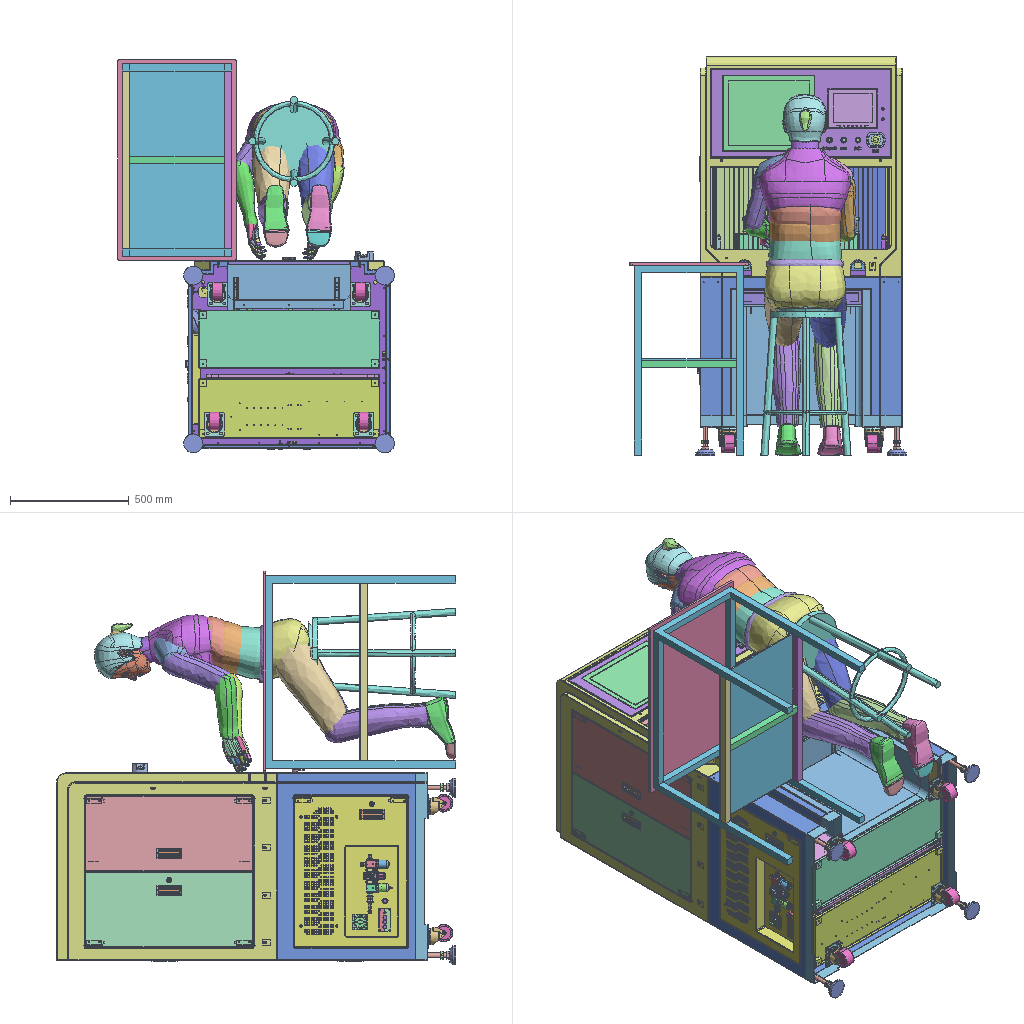Assembly | SolidWorks | 209 different items | 351 placed | box 1166 x 1682 x 1659 mm
Parts list (item | name | quantity | parent item | size | volume | features):
1 | (subassembly) | x1 | - | 263.704 x 74.5 x 59.5 mm | 261559 mm3 | -
2 | (subassembly) | x2 | in 6 | 37.5 x 724 x 636 mm | 879257 mm3 | -
3 | (subassembly) | x1 | in 6 | 37.5 x 764 x 737 mm | 1042688 mm3 | -
4 | (subassembly) | x1 | in 3 | 35.649 x 764 x 379.5 mm | 533274 mm3 | -
5 | (subassembly) | x1 | in 3 | 37.5 x 764 x 367.5 mm | 509414 mm3 | -
6 | (subassembly) | x1 | - | - | 7744813 mm3 | features ReferencePattern 9, LocalLPattern 2
7 | (subassembly) | x2 | in 2 | 35.649 x 724 x 329 mm | 451406 mm3 | -
8 | (subassembly) | x2 | in 2 | 37.5 x 724 x 317 mm | 427850 mm3 | -
9 | (subassembly) | x1 | - | - | 9143617 mm3 | features HoleWzd 1
10 | (subassembly) | x1 | in 9 | 37.5 x 494 x 636 mm | 633113 mm3 | -
11 | (subassembly) | x1 | - | - | 5781926 mm3 | -
12 | (subassembly) | x1 | in 9 | 37.5 x 494 x 731 mm | 708096 mm3 | -
13 | (subassembly) | x1 | - | 851.002 x 954.449 x 1522 mm | 114343551 mm3 | -
14 | (subassembly) | x2 | in 15 | 75 x 75 x 100.5 mm | 180032 mm3 | -
15 | (subassembly) | x1 | in 22 | - | 6635469 mm3 | features CompositeCurve 14, InContextFeatHolder 6, ReferencePattern 5, LocalLPattern 1
16 | (subassembly) | x1 | - | 27.5 x 27.5 x 50 mm | 15432 mm3 | -
17 | (subassembly) | x1 | - | 27.486 x 37 x 27.571 mm | 9512 mm3 | features AEMSimFeature 1
18 | (subassembly) | x1 | - | 27.486 x 37 x 27.571 mm | 9512 mm3 | features AEMSimFeature 1
19 | (subassembly) | x2 | - | 120.002 x 37.222 x 120.002 mm | 118437 mm3 | features AEMSimFeature 1
20 | (subassembly) | x1 | in 22 | - | 7028567 mm3 | -
21 | (subassembly) | x1 | in 20 | - | 7028567 mm3 | features InContextFeatHolder 12
22 | (subassembly) | x1 | - | - | 13967831 mm3 | -
23 | (subassembly) | x1 | in 21 | 66 x 382.5 x 279.882 mm | 1255947 mm3 | features CompositeCurve 1
24 | (subassembly) | x1 | in 25 | 120 x 120 x 447.19 mm | 1943055 mm3 | -
25 | (subassembly) | x1 | in 21 | 150 x 447.19 x 260.95 mm | 4314882 mm3 | features InContextFeatHolder 4, AEMSimFeature 1
26 | (subassembly) | x1 | - | 110 x 110 x 178 mm | 343146 mm3 | -
27 | (subassembly) | x1 | - | 212.5 x 110 x 178 mm | 375386 mm3 | -
28 | (subassembly) | x1 | - | 27.486 x 37 x 27.571 mm | 9512 mm3 | features AEMSimFeature 1
29 | (subassembly) | x1 | in 9 | 513 x 62 x 319 mm | 391027 mm3 | -
30 | (subassembly) | x1 | in 10 | 35.649 x 494 x 329 mm | 327464 mm3 | -
31 | (subassembly) | x1 | in 12 | 35.649 x 494 x 376.5 mm | 364955 mm3 | -
32 | (subassembly) | x1 | in 10 | 37.5 x 494 x 317 mm | 305649 mm3 | -
33 | (subassembly) | x1 | in 23 | 279.882 x 382.5 x 66 mm | 1255947 mm3 | -
34 | (subassembly) | x1 | in 12 | 37.5 x 494 x 364.5 mm | 343141 mm3 | -
35 | (subassembly) | x4 | in 9 | 82 x 108 x 101.5 mm | 268701 mm3 | -
36 | (subassembly) | x1 | in 33 | 129 x 145.682 x 60 mm | 347551 mm3 | -
37 | (subassembly) | x1 | - | - | - | features InContextFeatHolder 2
38 | (subassembly) | x2 | in 9 | 19.1 x 27 x 355.6 mm | 53806 mm3 | features AEMSimFeature 1
39 | (subassembly) | x1 | - | 62 x 132 x 147 mm | 286848 mm3 | -
40 | - | x1 | - | - | - | features RefSurface 13
41 | - | x2 | in 14 | 24 x 24 x 95 mm | 18042 mm3 | features ICE 4, Chamfer 3, HoleWzd 2, Extrusion 1
42 | - | x1 | - | 80 x 64 x 38.5 mm | 66365 mm3 | features BaseBody 1
43 | - | x1 | - | 40 x 40 x 73.5 mm | 58670 mm3 | features ICE 8, CirPattern 2, Chamfer 1, Extrusion 1, MirrorPattern 1, Revolution 1
44 | - | x1 | in 29 | 55 x 52.573 x 12.5 mm | 11112 mm3 | features BaseBody 1, HoleWzd 1
45 | - | x1 | - | 800 x 600 x 10 mm | 4796860 mm3 | features Extrusion 1, Fillet 1, HoleWzd 1
46 | - | x1 | - | 79 x 50 x 11.5 mm | 8238 mm3 | features EdgeFlange 4, HoleWzd 3, Fillet 2, FlatPattern 1, SMBaseFlange 1, SheetMetal 1
47 | - | x1 | in 15 | 40 x 120 x 200 mm | 151570 mm3 | features FlatPattern 1, HoleWzd 1, ICE 1, SMBaseFlange 1, SheetMetal 1
48 | - | x1 | in 15 | 200 x 30 x 20 mm | 113265 mm3 | features Extrusion 1, HoleWzd 1
49 | - | x1 | - | 16.166 x 14 x 25.5 mm | 2115 mm3 | features ICE 1, Revolution 1
50 | - | x1 | - | 16.5 x 51.05 x 30.583 mm | 7205 mm3 | features RevCut 2, Revolution 2, ICE 1
51 | - | x1 | - | - | - | features RefSurface 3
52 | - | x11 | in 4, 5, 7, 8, 9, 30, 31, 32, 34 | 26.5 x 89 x 10.2 mm | 8027 mm3 | features ICE 2, Chamfer 1, Sweep 1
53 | - | x10 | in 4, 7, 30, 31 | 42 x 30.3 x 68.3 mm | 12070 mm3 | features BaseBody 4
54 | - | x11 | in 4, 5, 7, 8, 9, 30, 31, 32, 34 | 26.5 x 89 x 10.2 mm | 8027 mm3 | features ICE 2, Chamfer 1, Sweep 1
55 | - | x4 | in 15 | 30 x 30 x 4.5 mm | 1696 mm3 | features Extrusion 1
56 | - | x4 | in 15 | 75 x 75 x 50 mm | 173343 mm3 | features HoleWzd 2, Extrusion 1, RevCut 1
57 | - | x1 | in 15 | 520 x 157 x 80 mm | 647127 mm3 | features ICE 2, SMWeldBead 2, Cut 1, EdgeFlange 1, Fillet 1, FlatPattern 1, HoleWzd 1, SMBaseFlange 1, SheetMetal 1
58 | - | x1 | in 15 | 520 x 157 x 80 mm | 639490 mm3 | features ICE 3, Cut 2, SMWeldBead 2, EdgeFlange 1, Fillet 1, FlatPattern 1, SMBaseFlange 1, SheetMetal 1
59 | - | x2 | in 15 | 25 x 25 x 420 mm | 181738 mm3 | features ICE 4, Chamfer 2, HoleWzd 2, Extrusion 1
60 | - | x1 | in 9 | 851 x 582 x 791 mm | 1784461 mm3 | features ICE 16, Fillet 6, HoleWzd 2, Extrusion 1, Shell 1
61 | - | x2 | - | 22 x 34 x 300 mm | 181288 mm3 | features Extrusion 1
62 | - | x1 | - | 16 x 1.6 x 16 mm | 219.911 mm3 | features Revolution 1
63 | - | x4 | in 6 | 26.5 x 60 x 14.5 mm | 2856 mm3 | features ICE 2, Chamfer 1, FlatPattern 1, SMBaseFlange 1, SheetMetal 1
64 | - | x2 | in 6 | 378 x 24.5 x 30 mm | 18043 mm3 | features ICE 2, Chamfer 1, FlatPattern 1, SMBaseFlange 1, SheetMetal 1
65 | - | x1 | - | 270 x 29.5 x 60 mm | 28669 mm3 | features ICE 2, Chamfer 1, FlatPattern 1, HoleWzd 1, SMBaseFlange 1, SheetMetal 1
66 | - | x1 | in 6 | 758 x 373 x 23.5 mm | 379988 mm3 | features ICE 12, HoleWzd 3, Fillet 2, Extrusion 1, Shell 1
67 | - | x1 | in 9 | 638 x 478 x 53 mm | 589173 mm3 | features ICE 16, Fillet 4, HoleWzd 4, LPattern 4, Cut 1, Extrusion 1
68 | - | x1 | in 15 | 40 x 120 x 619.772 mm | 529398 mm3 | features ICE 3, Fillet 2, HoleWzd 2, Chamfer 1, EdgeFlange 1, FlatPattern 1, SMBaseFlange 1, SheetMetal 1
69 | - | x1 | in 15 | 40 x 120 x 619.772 mm | 529398 mm3 | features Fillet 2, HoleWzd 2, ICE 2, Chamfer 1, Cut 1, EdgeFlange 1, FlatPattern 1, SMBaseFlange 1, SheetMetal 1
70 | - | x1 | in 9 | 729 x 16 x 537 mm | 887754 mm3 | features HoleWzd 7, ICE 2, LPattern 2, EdgeFlange 1, FlatPattern 1, SMBaseFlange 1, SheetMetal 1
71 | - | x1 | - | 65.5 x 65.5 x 79 mm | 180207 mm3 | features ICE 6, Fillet 3, Chamfer 2, Extrusion 1, HoleWzd 1
72 | - | x1 | - | 24 x 27.713 x 43 mm | 10470 mm3 | features ICE 2, Extrusion 1, Fillet 1
73 | - | x1 | - | 12.277 x 12.254 x 2.1 mm | 135.755 mm3 | features Extrusion 1
74 | - | x2 | in 15 | 535 x 85 x 50 mm | 287832 mm3 | features Extrusion 1
75 | - | x1 | in 6 | 210 x 2 x 210 mm | 88000 mm3 | features Extrusion 1, Fillet 1, HoleWzd 1
76 | - | x1 | - | 40 x 100 x 160 mm | 100089 mm3 | features ICE 2, Chamfer 1, FlatPattern 1, SMBaseFlange 1, SheetMetal 1
77 | - | x1 | - | 48 x 48 x 18 mm | 31644 mm3 | features Extrusion 1
78 | - | x1 | in 21 | 180 x 730 x 60 mm | 1457746 mm3 | features HoleWzd 5, Chamfer 1, Extrusion 1, ICE 1, MirrorPattern 1
79 | - | x11 | in 4, 5, 7, 8, 9, 30, 31, 32, 34 | 42.062 x 107.5 x 14.849 mm | 13665 mm3 | features BaseBody 3
80 | - | x6 | in 5, 8, 9, 32, 34 | 21.6 x 37.5 x 21.6 mm | 6258 mm3 | features BaseBody 1
81 | - | x1 | - | 110 x 110 x 178 mm | 318581 mm3 | features ICE 2, MirrorPattern 1, RevCut 1, Revolution 1
82 | - | x1 | - | 160 x 60 x 10 mm | 92142 mm3 | features HoleWzd 2, Extrusion 1
83 | - | x1 | - | - | - | features RefSurface 5
84 | - | x1 | - | 45 x 45 x 500 mm | 317021 mm3 | features Extrusion 1, HoleWzd 1
85 | - | x2 | in 15 | 25 x 13 x 25 mm | 3768 mm3 | features Extrusion 1
86 | - | x1 | in 25 | 92 x 60 x 144 mm | 769072 mm3 | features HoleWzd 2, Chamfer 1, Extrusion 1
87 | - | x1 | in 25 | 140 x 390.5 x 15 mm | 813690 mm3 | features HoleWzd 7, Extrusion 1, Fillet 1, ICE 1
88 | - | x1 | in 15 | 30 x 20 x 30 mm | 7536 mm3 | features Extrusion 1
89 | - | x2 | in 6 | 825 x 30 x 22 mm | 48151 mm3 | features ICE 3, Chamfer 1, Extrusion 1, Fillet 1, HoleWzd 1
90 | - | x1 | - | 590 x 1000 x 5 mm | 2949750 mm3 | features Chamfer 1, Extrusion 1
91 | - | x1 | - | 790 x 1000 x 5 mm | 3949750 mm3 | features Chamfer 1, Extrusion 1
92 | - | x8 | - | 20 x 6 x 6 mm | 537.381 mm3 | features RefAxis 3, 3DProfileFeature 1, RevCut 1, Revolution 1
93 | - | x2 | in 29 | 20 x 23.481 x 200 mm | 6904 mm3 | features BaseBody 1, ICE 1
94 | - | x1 | in 29 | 513 x 62 x 306.5 mm | 366101 mm3 | features ICE 9, Extrusion 1, Fillet 1, Shell 1
95 | - | x1 | - | 45 x 45 x 1000 mm | 638120 mm3 | features Extrusion 1
96 | - | x1 | in 30 | 20.237 x 477 x 329 mm | 273605 mm3 | features EdgeFlange 6, ICE 5, Chamfer 1, FlatPattern 1, SMBaseFlange 1, SheetMetal 1
97 | - | x1 | in 31 | 20.237 x 477 x 376.5 mm | 311097 mm3 | features EdgeFlange 6, ICE 5, Chamfer 1, FlatPattern 1, SMBaseFlange 1, SheetMetal 1
98 | - | x1 | in 32 | 15 x 477 x 317 mm | 269673 mm3 | features EdgeFlange 4, ICE 4, FlatPattern 1, SMBaseFlange 1, SheetMetal 1
99 | - | x1 | in 34 | 15 x 477 x 364.5 mm | 307164 mm3 | features EdgeFlange 4, ICE 4, FlatPattern 1, SMBaseFlange 1, SheetMetal 1
100 | - | x1 | in 33 | 15 x 17 x 15 mm | 2439 mm3 | features BaseBody 1
101 | - | x1 | in 9 | 475 x 165 x 2 mm | 114873 mm3 | features HoleWzd 2, Chamfer 1, Extrusion 1, ICE 1
102 | - | x1 | in 15 | 120 x 185 x 70 mm | 181748 mm3 | features ICE 6, Chamfer 3, Extrusion 1
103 | - | x1 | - | 45 x 45 x 700 mm | 446684 mm3 | features Extrusion 1
104 | - | x1 | - | 45 x 45 x 545 mm | 347775 mm3 | features Extrusion 1
105 | - | x2 | in 19 | 120.002 x 37.222 x 120.002 mm | 72632 mm3 | features BaseBody 1, ICE 1, Scale 1
106 | - | x1 | in 15 | 90 x 200 x 90 mm | 1142205 mm3 | features ICE 6, Fillet 2, CirPattern 1, Extrusion 1, HoleWzd 1, RefAxis 1
107 | - | x1 | in 33 | 105 x 90 x 52.5 mm | 149012 mm3 | features BaseBody 1
108 | - | x1 | in 22 | 405 x 150 x 5 mm | 303750 mm3 | features Extrusion 1
109 | - | x1 | in 24 | 74 x 74 x 66.99 mm | 341850 mm3 | features BaseBody 24
110 | - | x1 | in 24 | 384.7 x 120 x 120 mm | 1601205 mm3 | features BaseBody 1, ICE 1
111 | - | x2 | in 19 | - | - | features RefSurface 1, Scale 1
112 | - | x2 | in 15 | 66 x 13 x 42 mm | 15219 mm3 | features ICE 3, Fillet 2, Extrusion 1
113 | - | x4 | in 14 | 11 x 35 x 35 mm | 5288 mm3 | features Revolution 6, CirPattern 2, RevCut 2, MirrorPattern 1
114 | - | x2 | in 39 | 40.25 x 51.3 x 11.5 mm | 9114 mm3 | features RefAxis 12, ICE 6, 3DProfileFeature 4, RevCut 2, Extrusion 1, Revolution 1
115 | - | x1 | in 39 | 23.253 x 8.6 x 25 mm | 822.627 mm3 | features RefAxis 3, ICE 2, 3DProfileFeature 1, Revolution 1
116 | - | x1 | in 39 | 40 x 61.6 x 47 mm | 55419 mm3 | features ICE 20, RefAxis 12, 3DProfileFeature 4, RevCut 3, Extrusion 1, Revolution 1
117 | - | x1 | in 39 | 36 x 81 x 36 mm | 24193 mm3 | features RefAxis 3, Revolution 2, 3DProfileFeature 1, ICE 1
118 | - | x2 | in 38 | 9.344 x 19.967 x 355.6 mm | 18790 mm3 | features BaseBody 1, RefAxis 1
119 | - | x1 | in 39 | 18 x 23.5 x 18 mm | 1546 mm3 | features RefAxis 6, 3DProfileFeature 2, Revolution 1
120 | - | x2 | in 39 | 4.9 x 38.3 x 11.5 mm | 1758 mm3 | features RefAxis 9, 3DProfileFeature 3, RevCut 2, Extrusion 1, ICE 1
121 | - | x4 | in 39 | 11 x 7 x 7 mm | 216.302 mm3 | features RefAxis 3, 3DProfileFeature 1, ICE 1, Revolution 1
122 | - | x1 | in 39 | 40 x 110.1 x 47 mm | 56293 mm3 | features ICE 40, RefAxis 9, 3DProfileFeature 3, RevCut 3, Extrusion 1, Revolution 1
123 | - | x1 | in 39 | 36 x 68 x 36 mm | 23842 mm3 | features RefAxis 3, 3DProfileFeature 1, ICE 1, Revolution 1
124 | - | x1 | in 17 | 25 x 37 x 25 mm | 9217 mm3 | features ICE 10, Fillet 2, LPattern 1, Revolution 1
125 | - | x1 | in 18 | 25 x 37 x 25 mm | 9217 mm3 | features ICE 10, Fillet 2, LPattern 1, Revolution 1
126 | - | x2 | in 17, 18 | 26.237 x 28.287 x 2 mm | 294.878 mm3 | features Extrusion 1
127 | - | x1 | in 39 | 15 x 27.1 x 27.1 mm | 10099 mm3 | features ICE 16, RefAxis 9, 3DProfileFeature 3, RevCut 2, Extrusion 1, Revolution 1
128 | - | x1 | in 39 | 40 x 43 x 47 mm | 55436 mm3 | features ICE 27, RefAxis 15, 3DProfileFeature 5, RevCut 2, Extrusion 1, LPattern 1, Revolution 1
129 | - | x1 | in 25 | 150 x 181 x 35 mm | 751527 mm3 | features HoleWzd 2, ICE 2, Chamfer 1, Extrusion 1, Fillet 1
130 | - | x1 | in 39 | 37 x 6.5 x 35.922 mm | 2594 mm3 | features RefAxis 3, 3DProfileFeature 1, ICE 1, Revolution 1
131 | - | x4 | in 39 | 5.512 x 5.512 x 9.5 mm | 81.226 mm3 | features RefAxis 3, 3DProfileFeature 1, ICE 1, Revolution 1
132 | - | x2 | in 39 | 4.984 x 5 x 17.2 mm | 126.363 mm3 | features RefAxis 3, 3DProfileFeature 1, ICE 1, Revolution 1
133 | - | x1 | in 39 | 40 x 46 x 38 mm | 33356 mm3 | features RefAxis 18, ICE 10, 3DProfileFeature 6, Extrusion 1, RevCut 1, Revolution 1
134 | - | x4 | in 39 | 5.5 x 5.5 x 1 mm | 15.412 mm3 | features RefAxis 3, 3DProfileFeature 1, ICE 1, Revolution 1
135 | - | x4 | in 35 | 51 x 75 x 75 mm | 191030 mm3 | features BaseBody 1
136 | - | x4 | in 35 | 82 x 12 x 100 mm | 48810 mm3 | features BaseBody 1
137 | - | x4 | in 35 | 70 x 68.5 x 74 mm | 29160 mm3 | features BaseBody 1
138 | - | x1 | in 1 | 59.5 x 68.85 x 59.5 mm | 56089 mm3 | features ICE 7, Fillet 2, CirPattern 1, Extrusion 1, RevCut 1
139 | - | x1 | in 1 | 50 x 253.304 x 50 mm | 205470 mm3 | features ICE 9, Fillet 2, LPattern 2, Chamfer 1, Dome 1, Extrusion 1, RevCut 1
140 | - | x1 | in 25 | 150 x 64.95 x 35 mm | 37539 mm3 | features Chamfer 1, Extrusion 1, Fillet 1, HoleWzd 1, ICE 1
141 | - | x1 | in 16 | 19.63 x 17.35 x 50 mm | 8637 mm3 | features RefAxis 3, 3DProfileFeature 1, ICE 1, Revolution 1
142 | - | x1 | in 16 | 27.5 x 27.5 x 30 mm | 6795 mm3 | features RefAxis 3, 3DProfileFeature 1, Revolution 1
143 | - | x3 | in 33 | 13.7 x 28.4 x 26 mm | 1939 mm3 | features BaseBody 1
144 | - | x1 | in 33 | 7 x 16 x 25.5 mm | 463.296 mm3 | features BaseBody 1
145 | - | x1 | in 33 | 191 x 44 x 63 mm | 28771 mm3 | features BaseBody 1
146 | - | x1 | in 33 | 188 x 63 x 12 mm | 94885 mm3 | features BaseBody 1
147 | - | x1 | in 33 | 104 x 334 x 40 mm | 423472 mm3 | features BaseBody 1
148 | - | x1 | in 33 | 82.5 x 334 x 8.7 mm | 80216 mm3 | features BaseBody 1
149 | - | x1 | in 33 | 102 x 62.7 x 5 mm | 28999 mm3 | features BaseBody 1
150 | - | x1 | in 33 | 74.5 x 16 x 45 mm | 40163 mm3 | features BaseBody 1
151 | - | x2 | in 38 | 9 x 27 x 355.6 mm | 7594 mm3 | features BaseBody 1, RefAxis 1
152 | - | x1 | in 33 | 74.5 x 23 x 45 mm | 54150 mm3 | features BaseBody 1
153 | - | x1 | in 28 | 26.237 x 28.287 x 2 mm | 294.878 mm3 | features Extrusion 1
154 | - | x1 | in 28 | 25 x 37 x 25 mm | 9217 mm3 | features ICE 10, Fillet 2, LPattern 1, Revolution 1
155 | - | x1 | - | 38.971 x 25 x 45 mm | 24565 mm3 | features Extrusion 1, MirrorPattern 1, RevCut 1
156 | - | x1 | - | 100 x 25 x 5 mm | 10800 mm3 | features Fillet 2, Extrusion 1, HoleWzd 1, ICE 1
157 | - | x1 | - | 100 x 25 x 5 mm | 10800 mm3 | features Fillet 2, Extrusion 1, HoleWzd 1, ICE 1
158 | - | x3 | - | 60 x 42 x 30 mm | 30390 mm3 | features Fillet 2, ICE 2, Chamfer 1, Extrusion 1, HoleWzd 1
159 | - | x1 | - | 384 x 316.5 x 50 mm | 4529826 mm3 | features ICE 2, Chamfer 1, CutThin 1, Extrusion 1, HoleWzd 1, MoveFace 1
160 | - | x1 | - | 202 x 162 x 40 mm | 1013492 mm3 | features BaseBody 1
161 | - | x4 | in 9 | - | - | features RefSurface 3
162 | - | x2 | in 38 | 9 x 27 x 355.6 mm | 7594 mm3 | features BaseBody 1, RefAxis 1
163 | - | x1 | in 36 | 6 x 28.381 x 6 mm | 414.888 mm3 | features BaseBody 1
164 | - | x1 | in 36 | 27.962 x 30.887 x 22.9 mm | 4595 mm3 | features BaseBody 1
165 | - | x1 | in 36 | 45.598 x 29.85 x 36 mm | 13881 mm3 | features BaseBody 1
166 | - | x1 | in 36 | 7.8 x 34.633 x 7.8 mm | 896.959 mm3 | features BaseBody 1
167 | - | x1 | in 36 | 23.7 x 19 x 14.5 mm | 1788 mm3 | features BaseBody 1
168 | - | x1 | in 36 | 129 x 60 x 60 mm | 324718 mm3 | features BaseBody 1
169 | - | x1 | in 36 | 23.7 x 14.55 x 11.2 mm | 1255 mm3 | features BaseBody 1
170 | - | x1 | in 4 | 20.237 x 747 x 379.5 mm | 479415 mm3 | features EdgeFlange 6, ICE 5, Chamfer 1, FlatPattern 1, SMBaseFlange 1, SheetMetal 1
171 | - | x1 | in 5 | 15 x 747 x 367.5 mm | 473438 mm3 | features EdgeFlange 4, ICE 4, FlatPattern 1, SMBaseFlange 1, SheetMetal 1
172 | - | x1 | in 6 | 851 x 930 x 791 mm | 4286500 mm3 | features ICE 38, Fillet 16, HoleWzd 10, Chamfer 1, Cut 1, Extrusion 1, LPattern 1, Shell 1
173 | - | x2 | in 38 | 7.8 x 26 x 355.6 mm | 9914 mm3 | features BaseBody 1, RefAxis 1
174 | - | x2 | in 7 | 20.237 x 707 x 329 mm | 397548 mm3 | features EdgeFlange 6, ICE 5, Chamfer 1, FlatPattern 1, SMBaseFlange 1, SheetMetal 1
175 | - | x2 | in 8 | 15 x 707 x 317 mm | 391874 mm3 | features EdgeFlange 4, ICE 4, FlatPattern 1, SMBaseFlange 1, SheetMetal 1
176 | - | x2 | in 15 | 75 x 75 x 50 mm | 180356 mm3 | features HoleWzd 2, Extrusion 1, ICE 1, RevCut 1
177 | - | x2 | in 14 | 24 x 5 x 24 mm | 1909 mm3 | features Chamfer 1, Extrusion 1, HoleWzd 1
178 | - | x1 | in 15 | 20 x 20 x 448 mm | 119242 mm3 | features ICE 5, Chamfer 1, Cut 1, Extrusion 1
179 | - | x1 | in 15 | 25.008 x 57.316 x 57.728 mm | 22409 mm3 | features HoleWzd 2, Chamfer 1, CirPattern 1, Cut 1, Fillet 1, ICE 1, Revolution 1
180 | - | x1 | in 15 | 25.008 x 57.316 x 57.728 mm | 22718 mm3 | features HoleWzd 2, ICE 2, Chamfer 1, CirPattern 1, Cut 1, Fillet 1, Revolution 1
181 | - | x3 | - | 26 x 27.999 x 7 mm | 2114 mm3 | features ICE 4, Dome 1, Extrusion 1
182 | - | x16 | in 6 | 33 x 33 x 25 mm | 2832 mm3 | features ICE 2, Extrusion 1, Fillet 1
183 | - | x1 | in 13 | - | - | features RefSurface 71
184 | - | x2 | in 38 | 7.8 x 26 x 355.6 mm | 9914 mm3 | features BaseBody 1, RefAxis 1
185 | - | x1 | - | 817 x 20 x 757 mm | 11961283 mm3 | features HoleWzd 10, ICE 5, LPattern 2, Extrusion 1, Fillet 1
186 | - | x2 | - | 22 x 290 x 232.8 mm | 181561 mm3 | features ICE 3, Extrusion 1, LPattern 1, MirrorPattern 1, Revolution 1
187 | - | x2 | - | 22 x 450 x 232.8 mm | 289994 mm3 | features ICE 3, Extrusion 1, LPattern 1, MirrorPattern 1, Revolution 1
188 | - | x1 | in 9 | 589 x 380 x 530 mm | 943074 mm3 | features ICE 9, Fillet 6, HoleWzd 3, Cut 2, ExtruThin 1
189 | - | x1 | in 13 | 850 x 500 x 810 mm | 12634142 mm3 | features ICE 6, Extrusion 1, Fillet 1
190 | - | x2 | in 14 | 75 x 75 x 50 mm | 149506 mm3 | features ICE 2, Extrusion 1, RevCut 1
191 | - | x1 | in 9 | 851 x 50 x 791 mm | 311497 mm3 | features ICE 7, Fillet 5, Extrusion 1, Shell 1
192 | - | x1 | in 9 | 764 x 16 x 252 mm | 477309 mm3 | features HoleWzd 6, LPattern 3, EdgeFlange 1, FlatPattern 1, ICE 1, SMBaseFlange 1, SheetMetal 1
193 | - | x1 | in 9 | 764 x 16 x 244.5 mm | 466147 mm3 | features EdgeFlange 1, FlatPattern 1, HoleWzd 1, ICE 1, SMBaseFlange 1, SheetMetal 1
194 | - | x2 | in 15 | 85 x 45 x 15 mm | 38919 mm3 | features Chamfer 1, Extrusion 1, HoleWzd 1, ICE 1
195 | - | x1 | in 15 | 64.757 x 208.466 x 16.625 mm | 48801 mm3 | features Boss 3, CurvePattern 2, Chamfer 1, CompositeCurve 1, Extrusion 1, MirrorPattern 1, MirrorSolid 1
196 | hex lobular socket head cap screws-8.8 gb | x1 | - | - | - | -
197 | hex thin nuts-grades ab-chamfered gb | x1 | - | - | - | -
198 | plain washers--product grade c gb | x1 | - | - | - | -
199 | spring lock washers--normal type gb | x1 | - | - | - | -
200 | Side Plate-1 | x1 | - | - | - | -
201 | Side Plate-2 | x1 | - | - | - | -
202 | Side Plate-3 | x1 | - | - | - | -
203 | Bottom Cover Plate | x1 | - | - | - | -
204 | Square Tube 1 | x1 | - | - | - | -
205 | Square Tube 5 | x1 | - | - | - | -
206 | Square Tube 6 | x1 | - | - | - | -
207 | Square Tube 7 | x1 | - | - | - | -
208 | Square Tube Welded Frame | x1 | - | - | - | -
209 | Leveling Feet and Casters (subassembly) | x1 | - | - | - | -
Mates (type | each side: item.copy, entity, surface, feature), first 465 of 568 lines:
In the top assembly
Concentric | 185.1 face cylinder M3 Tapped Hole 3 | 181.1 face cylinder Extrude 3 | 2 times
Concentric | 185.1 face cylinder M3 Tapped Hole 3 | 181.2 face cylinder Extrude 3 | 2 times
Coordinate | 185.1 select_type:25 | assembly select_type:11
Coincident | 185.1 face plane Boss-Extrude 1 | 181.3 face plane Extrude 1
Coincident | 185.1 face plane Boss-Extrude 1 | 158.1 face plane Extrude 1
Concentric | 185.1 face cylinder M5 Tapped Hole 2 | 158.1 face cylinder M5 Hex Socket Head Cap Screw Counterbore Hole 1 | 2 times
Width | 181.3 face plane Extrude 1 | 181.3 face plane Extrude 1 | 158.1 face plane Extrude 3 | 158.1 face plane Extrude 3
Concentric | 185.1 face cylinder M3 Tapped Hole 3 | 181.3 face cylinder Extrude 3
Coincident | 185.1 face plane Boss-Extrude 1 | 158.2 face plane Extrude 1
Concentric | 185.1 face cylinder M5 Tapped Hole 2 | 158.2 face cylinder M5 Hex Socket Head Cap Screw Counterbore Hole 1 | 2 times
Coincident | 185.1 face plane Boss-Extrude 1 | 181.1 face plane Extrude 1
Coincident | 185.1 face plane Boss-Extrude 1 | 158.3 face plane Extrude 1
Concentric | 185.1 face cylinder M5 Tapped Hole 2 | 158.3 face cylinder M5 Hex Socket Head Cap Screw Counterbore Hole 1 | 2 times
Coincident | 185.1 face plane Boss-Extrude 1 | 181.2 face plane Extrude 1
Concentric | 185.1 face cylinder Ø6.0 (6) DiameterHole 1 | 92.1 face cylinder Revolve 1
Concentric | 185.1 face cylinder Ø6.0 (6) DiameterHole 1 | 92.2 face cylinder Revolve 1
Concentric | 185.1 face cylinder Ø6.0 (6) DiameterHole 1 | 92.3 face cylinder Revolve 1
Concentric | 185.1 face cylinder Ø6.0 (6) DiameterHole 1 | 92.4 face cylinder Revolve 1
Concentric | 185.1 face cylinder Ø6.0 (6) DiameterHole 2 | 92.5 face cylinder Revolve 1
Concentric | 185.1 face cylinder Ø6.0 (6) DiameterHole 2 | 92.6 face cylinder Revolve 1
Concentric | 185.1 face cylinder Ø6.0 (6) DiameterHole 2 | 92.7 face cylinder Revolve 1
Concentric | 185.1 face cylinder Ø6.0 (6) DiameterHole 2 | 92.8 face cylinder Revolve 1
Coincident | 92.3 face plane Revolve 1 | 92.4 face plane Revolve 1
Coincident | 92.1 face plane Revolve 1 | 92.2 face plane Revolve 1
Coincident | 92.7 face plane Revolve 1 | 92.8 face plane Revolve 1
Coincident | 92.5 face plane Revolve 1 | 92.6 face plane Revolve 1
Coincident | 60.1 face plane | 172.1 face plane Boss-Extrude 1 | 2 times
Coincident | 60.1 face plane | 172.1 face plane Boss-Extrude 2
Coincident | 66.1 face plane Boss-Extrude 1 | 42.1 face plane Import 1
Concentric | 66.1 face cylinder Cut-Extrude 5 | 43.1 face cylinder Boss-Extrude 3
Coincident | 66.1 face plane Boss-Extrude 1 | 43.1 face plane Boss-Extrude 1
Concentric | 43.1 face cylinder Boss-Extrude 1 | 42.1 face cylinder Import 1
Concentric | 66.1 face cylinder Cut-Extrude 5 | 125.1 face cylinder Revolve 1
Coincident | 66.1 face plane Boss-Extrude 1 | 125.1 face plane Revolve 1
Concentric | 66.1 face cylinder Cut-Extrude 5 | 124.1 face cylinder Revolve 1
Coincident | 66.1 face plane Boss-Extrude 1 | 124.1 face plane Revolve 1
Concentric | 66.1 face cylinder Cut-Extrude 5 | 154.1 face cylinder Revolve 1
Coincident | 66.1 face plane Boss-Extrude 1 | 154.1 face plane Revolve 1
Coincident | 186.1 face plane Mirror 1 | 186.2 face plane Mirror 1
Coincident | 186.1 face plane Extrude 3 | 186.2 face plane Extrude 3
Coincident | 186.2 face plane Extrude 1 | 187.1 face plane Extrude 1 | 3 times
Coincident | 186.2 face plane Extrude 3 | 89.1 face plane Boss-Extrude 1
Coincident | 187.1 face plane Extrude 3 | 187.2 face plane Extrude 3
Coincident | 187.1 face plane Mirror 1 | 187.2 face plane Mirror 1
Coincident | 187.2 face plane Extrude 1 | 186.1 face plane Extrude 1
Coincident | 187.2 face plane Extrude 3 | 89.2 face plane Boss-Extrude 1
Width | 187.2 face plane Mirror 1 | 186.1 face plane Mirror 1 | 172.1 face plane Shell 1 | 172.1 face plane Shell 1
Width | 186.1 face plane Extrude 3 | 186.1 face plane Extrude 3 | 89.2 face plane Boss-Extrude 1 | 89.2 face plane Boss-Extrude 1
Coincident | 114.1 face plane Boss-Extrude 1 | 67.1 face plane Boss-Extrude 5
Width | 114.2 face plane Cut-Extrude 1 | 114.2 face plane Cut-Extrude 1 | 67.1 face cylinder M5 Tapped Hole 1
Width | 114.1 face plane Cut-Extrude 1 | 114.1 face plane Cut-Extrude 1 | 67.1 face cylinder M5 Tapped Hole 1
DistanceDim | 50.1 face plane Revolve 2 | 141.1 face plane Revolve 1
Concentric | 141.1 face cylinder Revolve 1 | 50.1 face cylinder Revolve 2
Coincident | 116.1 face plane Boss-Extrude 7 | 141.1 face plane Revolve 1
Concentric | 116.1 face cylinder Cut-Revolve 2 | 141.1 face cylinder Revolve 1
Concentric | 72.1 face cylinder Boss-Extrude 4 | 67.1 face cylinder Cut-Extrude 8
Coincident | 72.1 face plane Boss-Extrude 1 | 67.1 face plane Boss-Extrude 5
Concentric | 49.1 face cylinder Revolve 1 | 67.1 face cylinder Cut-Extrude 9
Coincident | 122.1 face plane Boss-Extrude 5 | 49.1 face plane Revolve 1
Concentric | 122.1 edge | 49.1 face cylinder Revolve 1
Coincident | 71.1 face plane Boss-Extrude 5 | 67.1 face plane Boss-Extrude 5
Concentric | 71.1 face cylinder M4 Tapped Hole 1 | 67.1 face cylinder Ø4.5 (4.5) DiameterHole 1 | 2 times
Coincident | 105.1 face plane Import 1 | 101.1 face plane Boss-Extrude 1
Concentric | 105.1 face cylinder Cut-Extrude 1 | 101.1 face cylinder M4 Tapped Hole 1 | 2 times
Coincident | 105.2 face plane Import 1 | 101.1 face plane Boss-Extrude 1
Concentric | 105.2 face cylinder Cut-Extrude 1 | 101.1 face cylinder M4 Tapped Hole 1 | 2 times
Coincident | 66.1 face plane Boss-Extrude 4 | 159.1 face plane Cut-Extrude-Thin 1
Width | 159.1 face plane Boss-Extrude 1 | 159.1 face plane Boss-Extrude 1 | 66.1 face plane Cut-Extrude 2 | 66.1 face plane Cut-Extrude 2
Width | 66.1 face plane Cut-Extrude 2 | 66.1 face plane Cut-Extrude 2 | 159.1 face plane Boss-Extrude 1 | 159.1 face plane Boss-Extrude 1
Coincident | 159.1 face plane Boss-Extrude 1 | 64.1 face plane Base-Flange 1
Width | 64.1 face plane Cut-Extrude 1 | 64.1 face plane Cut-Extrude 1 | 159.1 face cylinder M5 Tapped Hole 1
Coincident | 159.1 face plane Boss-Extrude 1 | 64.2 face plane Base-Flange 1
Width | 64.2 face plane Cut-Extrude 1 | 64.2 face plane Cut-Extrude 1 | 159.1 face cylinder M5 Tapped Hole 1
Concentric | 156.1 face cylinder M3 Hex Socket Countersunk Screw Countersink Hole 1 | 67.1 face cylinder M3 Tapped Hole 1 | 2 times
Coincident | 156.1 face plane Boss-Extrude 1 | 67.1 face plane Boss-Extrude 5
Coincident | 157.1 face plane Boss-Extrude 1 | 67.1 face plane Boss-Extrude 5
Concentric | 157.1 face cylinder M3 Hex Socket Countersunk Screw Countersink Hole 1 | 67.1 face cylinder M3 Tapped Hole 1 | 2 times
Coincident | 63.1 face plane Base-Flange 1 | 61.1 face plane Boss-Extrude 1 | 3 times
Coincident | 61.1 face plane Boss-Extrude 1 | 63.2 face plane Base-Flange 1 | 2 times
Coincident | 61.2 face plane Boss-Extrude 1 | 63.3 face plane Base-Flange 1 | 3 times
Coincident | 63.4 face plane Base-Flange 1 | 61.2 face plane Boss-Extrude 1 | 3 times
Coincident | 185.1 face cone Ø6.0 (6) DiameterHole 2 | 92.6 edge
Coincident | 185.1 face cone Ø6.0 (6) DiameterHole 2 | 92.8 edge
Coincident | 185.1 face cone Ø6.0 (6) DiameterHole 1 | 92.3 edge
Coincident | 185.1 face cone Ø6.0 (6) DiameterHole 1 | 92.2 edge
Width | 160.1 face plane Import 1 | 160.1 face plane Import 1 | 66.1 face plane Cut-Extrude 3 | 66.1 face plane Cut-Extrude 3 | 2 times
Coincident | 66.1 face plane Boss-Extrude 6 | 160.1 face plane Import 1
Coincident | 66.1 face plane Boss-Extrude 7 | 65.1 face plane Base-Flange 1
Width | 65.1 face plane Base-Flange 1 | 65.1 face plane Base-Flange 1 | 66.1 face plane Cut-Extrude 3 | 66.1 face plane Cut-Extrude 3
DistanceDim | 65.1 face plane Base-Flange 1 | 66.1 face plane Boss-Extrude 5
Concentric | 172.1 face cylinder Cut-Extrude 9 | 138.1 face cone Boss-Extrude 1
Parallel | 172.1 face plane Boss-Extrude 1 | 139.1 face plane Boss-Extrude 9
Coincident | 172.1 face plane Boss-Extrude 33 | 138.1 face plane Boss-Extrude 1
Coincident | 185.1 face plane Boss-Extrude 1 | 58.1 face plane Base-Flange 1
Width | 172.1 face plane Boss-Extrude 3 | 172.1 face plane Boss-Extrude 2 | 68.1 face plane Base-Flange 1 | 69.1 face plane Base-Flange 1
DistanceDim | 57.1 face plane Base-Flange 1 | 172.1 face plane Boss-Extrude 1
Coincident | 161.1 face plane HI_WAL01-D80-M20-L125-001-1-surface2 | 183.1 face plane SS03-1-surface1
Coincident | 172.1 face plane Boss-Extrude 1 | 189.1 face plane Boss-Extrude 1
In subassembly 6
Width | 66.2 face plane Boss-Extrude 1 | 66.2 face plane Boss-Extrude 1 | 172.2 face plane Cut-Extrude 2 | 172.2 face plane Cut-Extrude 2
Width | 172.2 face plane Cut-Extrude 2 | 172.2 face plane Cut-Extrude 2 | 66.2 face plane Boss-Extrude 1 | 66.2 face plane Boss-Extrude 1
Coincident | 172.2 face plane Boss-Extrude 4 | 64.3 face plane Base-Flange 1
Coincident | 172.2 face plane Boss-Extrude 4 | 64.4 face plane Base-Flange 1
Width | 172.2 face plane Cut-Extrude 3 | 172.2 face plane Cut-Extrude 3 | 175.1 face plane Edge-Flange 3 | 174.1 face plane Edge-Flange 3
Width | 172.2 face plane Cut-Extrude 3 | 172.2 face plane Cut-Extrude 3 | 175.1 face plane Edge-Flange 1 | 175.1 face plane Edge-Flange 1
Coincident | 172.2 face plane Boss-Extrude 10 | 175.2 face plane Edge-Flange 5
Width | 172.2 face plane Cut-Extrude 4 | 172.2 face plane Cut-Extrude 4 | 174.2 face plane Edge-Flange 3 | 175.2 face plane Edge-Flange 3
Width | 172.2 face plane Cut-Extrude 4 | 172.2 face plane Cut-Extrude 4 | 175.2 face plane Edge-Flange 1 | 175.2 face plane Edge-Flange 1
Coincident | 172.2 face plane Boss-Extrude 12 | 170.1 face plane Edge-Flange 5
Width | 170.1 face plane Edge-Flange 3 | 171.1 face plane Edge-Flange 3 | 172.2 face plane Cut-Extrude 5 | 172.2 face plane Cut-Extrude 5
Width | 170.1 face plane Edge-Flange 1 | 170.1 face plane Edge-Flange 1 | 172.2 face plane Cut-Extrude 5 | 172.2 face plane Cut-Extrude 5
Coincident | 172.2 face plane Boss-Extrude 8 | 175.1 face plane Edge-Flange 5
Coincident | 172.2 face plane Boss-Extrude 5 | 66.2 face plane Boss-Extrude 1
Width | 172.2 face plane Shell 1 | 172.2 face plane Shell 1 | 89.3 face plane Boss-Extrude 1 | 89.3 face plane Boss-Extrude 1
DistanceDim | 172.2 face plane Shell 1 | 89.3 face plane Boss-Extrude 1
Width | 89.3 face plane Cut-Extrude 1 | 89.3 face plane Cut-Extrude 1 | 172.2 face cylinder M4 Tapped Hole 1
Coincident | 89.3 face plane Boss-Extrude 1 | 89.4 face plane Boss-Extrude 1 | 2 times
Width | 89.4 face plane Cut-Extrude 1 | 89.4 face plane Cut-Extrude 1 | 172.2 face cylinder M4 Tapped Hole 1
Coincident | 63.5 face plane Base-Flange 1 | 63.6 face plane Base-Flange 1 | 2 times
Coincident | 172.2 face plane Boss-Extrude 18 | 63.6 face plane Base-Flange 1 | 2 times
Coincident | 172.2 face plane Boss-Extrude 18 | 63.7 face plane Base-Flange 1 | 2 times
Coincident | 172.2 face plane Boss-Extrude 18 | 63.8 face plane Base-Flange 1 | 3 times
Concentric | 172.2 face cylinder M4 Tapped Hole 5 | 75.1 face cylinder Ø5.0 (5) DiameterHole 1 | 2 times
Coincident | 172.2 face plane Shell 1 | 182.1 face plane Boss-Extrude 1
DistanceDim | 172.2 face plane Boss-Extrude 22 | 182.1 face plane Boss-Extrude 1
DistanceDim | 182.1 face plane Boss-Extrude 1 | 172.2 face plane Shell 1
Coincident | 172.2 face plane Shell 1 | 182.2 face plane Boss-Extrude 1
Coincident | 182.1 face plane Boss-Extrude 1 | 182.2 face plane Boss-Extrude 1 | 2 times
Coincident | 172.2 face plane Shell 1 | 182.3 face plane Boss-Extrude 1
Coincident | 182.4 face plane Boss-Extrude 1 | 182.3 face plane Boss-Extrude 1
DistanceDim | 182.3 face plane Boss-Extrude 1 | 172.2 face plane Shell 1
Coincident | 172.2 face plane Shell 1 | 182.5 face plane Boss-Extrude 1
Coincident | 182.2 face plane Boss-Extrude 1 | 182.5 face plane Boss-Extrude 1
DistanceDim | 172.2 face plane Shell 1 | 182.5 face plane Boss-Extrude 1
Coincident | 182.5 face plane Boss-Extrude 1 | 182.6 face plane Boss-Extrude 1
Coincident | 172.2 face plane Shell 1 | 182.6 face plane Boss-Extrude 1
DistanceDim | 182.6 face plane Boss-Extrude 1 | 182.5 face plane Boss-Extrude 1
Coincident | 172.2 face plane Boss-Extrude 1 | 75.1 face plane Boss-Extrude 1
Coincident | 182.5 face plane Boss-Extrude 1 | 182.7 face plane Boss-Extrude 1
Coincident | 172.2 face plane Shell 1 | 182.7 face plane Boss-Extrude 1
DistanceDim | 182.7 face plane Boss-Extrude 1 | 182.5 face plane Boss-Extrude 1
Coincident | 172.2 face plane Shell 1 | 182.8 face plane Boss-Extrude 1
Coincident | 182.6 face plane Boss-Extrude 1 | 182.8 face plane Boss-Extrude 1
DistanceDim | 182.8 face plane Boss-Extrude 1 | 182.6 face plane Boss-Extrude 1
Coincident | 63.8 face plane Base-Flange 1 | 63.7 face plane Base-Flange 1
Coincident | 63.5 face plane Base-Flange 1 | 63.7 face plane Base-Flange 1
In subassembly 2
Coincident | 174.3 face plane Base-Flange 1 | 175.3 face plane Base-Flange 1
DistanceDim | 175.3 face plane Edge-Flange 1 | 174.3 face plane Edge-Flange 6
Coincident | 174.3 face plane Edge-Flange 1 | 175.3 face plane Edge-Flange 1
In subassembly 8
Coincident | 175.4 face plane Base-Flange 1 | 79.1 face plane Import 3
Width | 79.1 face plane Import 3 | 79.1 face plane Import 3 | 175.4 face plane Cut-Extrude 5 | 175.4 face plane Cut-Extrude 5
Width | 79.1 face plane Import 3 | 79.1 face plane Import 2 | 175.4 face plane Cut-Extrude 5 | 175.4 face plane Cut-Extrude 5
Coincident | 175.4 face plane Base-Flange 1 | 54.1 face plane Boss-Extrude 1
DistanceDim | 175.4 face plane Edge-Flange 1 | 54.1 face plane Boss-Extrude 1
DistanceDim | 54.1 face plane Boss-Extrude 1 | 175.4 face plane Edge-Flange 3
Coincident | 175.4 face plane Base-Flange 1 | 52.1 face plane Boss-Extrude 1
Coincident | 54.1 face plane Boss-Extrude 1 | 52.1 face plane Boss-Extrude 1
DistanceDim | 52.1 face plane Boss-Extrude 1 | 175.4 face plane Edge-Flange 1
Concentric | 175.4 face cylinder Cut-Extrude 5 | 80.1 face cylinder Import 1
Coincident | 175.4 face plane Base-Flange 1 | 80.1 face plane Import 1
Parallel | 175.4 face plane Edge-Flange 5 | 80.1 face plane Import 1
In subassembly 7
Coincident | 174.4 face plane Base-Flange 1 | 79.1 face plane Import 3
Width | 79.1 face plane Import 3 | 79.1 face plane Import 3 | 174.4 face plane Cut-Extrude 5 | 174.4 face plane Cut-Extrude 5
Width | 79.1 face plane Import 3 | 79.1 face plane Import 2 | 174.4 face plane Cut-Extrude 5 | 174.4 face plane Cut-Extrude 5
Coincident | 174.4 face plane Base-Flange 1 | 53.1 face plane Import 9
Coincident | 174.4 face plane Edge-Flange 6 | 53.1 face plane Import 9
Coincident | 174.4 face plane Cut-Extrude 3 | 53.1 face plane Import 9
Coincident | 53.1 face plane Import 10 | 53.2 face plane Import 10
Coincident | 174.4 face plane Edge-Flange 6 | 53.2 face plane Import 9
Coincident | 174.4 face plane Cut-Extrude 3 | 53.2 face plane Import 9
Coincident | 174.4 face plane Base-Flange 1 | 54.1 face plane Boss-Extrude 1
DistanceDim | 174.4 face plane Edge-Flange 1 | 54.1 face plane Boss-Extrude 1
DistanceDim | 54.1 face plane Boss-Extrude 1 | 174.4 face plane Edge-Flange 3
Coincident | 174.4 face plane Base-Flange 1 | 52.1 face plane Boss-Extrude 1
Coincident | 54.1 face plane Boss-Extrude 1 | 52.1 face plane Boss-Extrude 1
DistanceDim | 52.1 face plane Boss-Extrude 1 | 174.4 face plane Edge-Flange 1
In subassembly 3
Coincident | 170.2 face plane Base-Flange 1 | 171.2 face plane Base-Flange 1
DistanceDim | 171.2 face plane Edge-Flange 1 | 170.2 face plane Edge-Flange 6
Coincident | 170.2 face plane Edge-Flange 1 | 171.2 face plane Edge-Flange 1
In subassembly 5
Coincident | 171.3 face plane Base-Flange 1 | 79.1 face plane Import 3
Width | 79.1 face plane Import 3 | 79.1 face plane Import 3 | 171.3 face plane Cut-Extrude 5 | 171.3 face plane Cut-Extrude 5
Width | 79.1 face plane Import 3 | 79.1 face plane Import 2 | 171.3 face plane Cut-Extrude 5 | 171.3 face plane Cut-Extrude 5
Coincident | 171.3 face plane Base-Flange 1 | 54.1 face plane Boss-Extrude 1
DistanceDim | 171.3 face plane Edge-Flange 1 | 54.1 face plane Boss-Extrude 1
DistanceDim | 54.1 face plane Boss-Extrude 1 | 171.3 face plane Edge-Flange 3
Coincident | 171.3 face plane Base-Flange 1 | 52.1 face plane Boss-Extrude 1
Coincident | 54.1 face plane Boss-Extrude 1 | 52.1 face plane Boss-Extrude 1
DistanceDim | 52.1 face plane Boss-Extrude 1 | 171.3 face plane Edge-Flange 1
Concentric | 171.3 face cylinder Cut-Extrude 5 | 80.1 face cylinder Import 1
Coincident | 171.3 face plane Base-Flange 1 | 80.1 face plane Import 1
Parallel | 171.3 face plane Edge-Flange 5 | 80.1 face plane Import 1
In subassembly 4
Coincident | 170.3 face plane Base-Flange 1 | 79.1 face plane Import 3
Width | 79.1 face plane Import 3 | 79.1 face plane Import 3 | 170.3 face plane Cut-Extrude 5 | 170.3 face plane Cut-Extrude 5
Width | 79.1 face plane Import 3 | 79.1 face plane Import 2 | 170.3 face plane Cut-Extrude 5 | 170.3 face plane Cut-Extrude 5
Coincident | 170.3 face plane Base-Flange 1 | 53.1 face plane Import 9
Coincident | 170.3 face plane Edge-Flange 6 | 53.1 face plane Import 9
Coincident | 170.3 face plane Cut-Extrude 3 | 53.1 face plane Import 9
Coincident | 53.1 face plane Import 10 | 53.2 face plane Import 10
Coincident | 170.3 face plane Edge-Flange 6 | 53.2 face plane Import 9
Coincident | 170.3 face plane Cut-Extrude 3 | 53.2 face plane Import 9
Coincident | 170.3 face plane Base-Flange 1 | 54.1 face plane Boss-Extrude 1
DistanceDim | 170.3 face plane Edge-Flange 1 | 54.1 face plane Boss-Extrude 1
DistanceDim | 54.1 face plane Boss-Extrude 1 | 170.3 face plane Edge-Flange 3
Coincident | 170.3 face plane Base-Flange 1 | 52.1 face plane Boss-Extrude 1
Coincident | 54.1 face plane Boss-Extrude 1 | 52.1 face plane Boss-Extrude 1
DistanceDim | 52.1 face plane Boss-Extrude 1 | 170.3 face plane Edge-Flange 1
In subassembly 9
Coincident | 188.1 face plane Extrude-Thin 1 | 60.2 face plane | 2 times
Width | 94.1 face plane Boss-Extrude 1 | 94.1 face plane Boss-Extrude 1 | 188.1 face plane Cut-Extrude 5 | 188.1 face plane Cut-Extrude 5
LimitDistanceDim | 188.1 face plane Boss-Extrude 10 | 94.1 face plane Boss-Extrude 1
Coincident | 188.1 face plane Boss-Extrude 10 | 162.1 face plane Import 1
Coincident | 188.1 face plane Boss-Extrude 10 | 162.2 face plane Import 1
Coincident | 162.1 face plane Import 1 | 162.2 face plane Import 1
DistanceDim | 151.1 face plane Import 1 | 151.2 face plane Import 1
DistanceDim | 151.1 face plane Import 1 | 94.1 face plane Boss-Extrude 2
Coincident | 151.2 face plane Import 1 | 94.1 face plane Boss-Extrude 2
Coincident | 96.1 face plane Edge-Flange 5 | 60.2 face plane
DistanceDim | 96.1 face plane Edge-Flange 1 | 60.2 face plane
DistanceDim | 96.1 face plane Edge-Flange 3 | 60.2 face plane
Coincident | 97.1 face plane Edge-Flange 5 | 60.2 face plane
DistanceDim | 97.1 face plane Edge-Flange 1 | 60.2 face plane
DistanceDim | 60.2 face plane | 97.1 face plane Edge-Flange 3
Coincident | 60.2 face plane | 191.1 face plane Boss-Extrude 1
Width | 67.2 face plane Boss-Extrude 1 | 67.2 face plane Boss-Extrude 1 | 60.2 face plane | 60.2 face plane
Width | 60.2 face plane | 60.2 face plane | 67.2 face plane Boss-Extrude 1 | 67.2 face plane Boss-Extrude 1
Coincident | 60.2 face plane | 67.2 face plane Boss-Extrude 2
Coincident | 67.2 face plane Boss-Extrude 1 | 79.1 face plane Import 3
Width | 79.1 face plane Import 3 | 79.1 face plane Import 3 | 67.2 face plane Cut-Extrude 4 | 67.2 face plane Cut-Extrude 4
Width | 67.2 face plane Cut-Extrude 4 | 67.2 face plane Cut-Extrude 4 | 79.1 face plane Import 2 | 79.1 face plane Import 3
Concentric | 67.2 face cylinder Cut-Extrude 3 | 80.1 face cylinder Import 1
Coincident | 67.2 face plane Boss-Extrude 1 | 80.1 face plane Import 1
Coincident | 67.2 face plane Boss-Extrude 1 | 52.1 face plane Boss-Extrude 1
Concentric | 67.2 face cylinder Cut-Extrude 1 | 52.1 face cylinder Sweep 1
DistanceDim | 52.1 face plane Boss-Extrude 1 | 67.2 face plane Boss-Extrude 2
Coincident | 67.2 face plane Boss-Extrude 1 | 54.1 face plane Boss-Extrude 1
Concentric | 67.2 face cylinder Cut-Extrude 2 | 54.1 face cylinder Sweep 1
DistanceDim | 54.1 face plane Boss-Extrude 1 | 67.2 face plane Boss-Extrude 3
Coincident | 67.2 face plane Boss-Extrude 6 | 101.2 face plane Boss-Extrude 1
Concentric | 67.2 face cylinder M4 Tapped Hole 1 | 101.2 face cylinder Ø5.0 (5) DiameterHole 1 | 2 times
Coincident | 161.2 face plane HI_WAL01-D80-M20-L125-001-1-surface2 | 161.3 face plane HI_WAL01-D80-M20-L125-001-1-surface2
Coincident | 161.3 face plane HI_WAL01-D80-M20-L125-001-1-surface2 | 161.4 face plane HI_WAL01-D80-M20-L125-001-1-surface2
Coincident | 161.4 face plane HI_WAL01-D80-M20-L125-001-1-surface2 | 161.5 face plane HI_WAL01-D80-M20-L125-001-1-surface2
In subassembly 10
Coincident | 96.2 face plane Base-Flange 1 | 98.1 face plane Base-Flange 1
DistanceDim | 98.1 face plane Edge-Flange 1 | 96.2 face plane Edge-Flange 6
Coincident | 96.2 face plane Edge-Flange 1 | 98.1 face plane Edge-Flange 1
In subassembly 30
Coincident | 96.3 face plane Base-Flange 1 | 79.1 face plane Import 3
Width | 79.1 face plane Import 3 | 79.1 face plane Import 3 | 96.3 face plane Cut-Extrude 5 | 96.3 face plane Cut-Extrude 5
Width | 79.1 face plane Import 3 | 79.1 face plane Import 2 | 96.3 face plane Cut-Extrude 5 | 96.3 face plane Cut-Extrude 5
Coincident | 96.3 face plane Base-Flange 1 | 53.1 face plane Import 9
Coincident | 96.3 face plane Edge-Flange 6 | 53.1 face plane Import 9
Coincident | 96.3 face plane Cut-Extrude 3 | 53.1 face plane Import 9
Coincident | 53.1 face plane Import 10 | 53.2 face plane Import 10
Coincident | 96.3 face plane Edge-Flange 6 | 53.2 face plane Import 9
Coincident | 96.3 face plane Cut-Extrude 3 | 53.2 face plane Import 9
Coincident | 96.3 face plane Base-Flange 1 | 54.1 face plane Boss-Extrude 1
DistanceDim | 96.3 face plane Edge-Flange 1 | 54.1 face plane Boss-Extrude 1
DistanceDim | 54.1 face plane Boss-Extrude 1 | 96.3 face plane Edge-Flange 3
Coincident | 96.3 face plane Base-Flange 1 | 52.1 face plane Boss-Extrude 1
Coincident | 54.1 face plane Boss-Extrude 1 | 52.1 face plane Boss-Extrude 1
DistanceDim | 52.1 face plane Boss-Extrude 1 | 96.3 face plane Edge-Flange 1
In subassembly 32
Coincident | 98.2 face plane Base-Flange 1 | 79.1 face plane Import 3
Width | 79.1 face plane Import 3 | 79.1 face plane Import 3 | 98.2 face plane Cut-Extrude 5 | 98.2 face plane Cut-Extrude 5
Width | 79.1 face plane Import 3 | 79.1 face plane Import 2 | 98.2 face plane Cut-Extrude 5 | 98.2 face plane Cut-Extrude 5
Coincident | 98.2 face plane Base-Flange 1 | 54.1 face plane Boss-Extrude 1
DistanceDim | 98.2 face plane Edge-Flange 1 | 54.1 face plane Boss-Extrude 1
DistanceDim | 54.1 face plane Boss-Extrude 1 | 98.2 face plane Edge-Flange 3
Coincident | 98.2 face plane Base-Flange 1 | 52.1 face plane Boss-Extrude 1
Coincident | 54.1 face plane Boss-Extrude 1 | 52.1 face plane Boss-Extrude 1
DistanceDim | 52.1 face plane Boss-Extrude 1 | 98.2 face plane Edge-Flange 1
Concentric | 98.2 face cylinder Cut-Extrude 5 | 80.1 face cylinder Import 1
Coincident | 98.2 face plane Base-Flange 1 | 80.1 face plane Import 1
Parallel | 98.2 face plane Edge-Flange 5 | 80.1 face plane Import 1
In subassembly 38
DistanceDim | 184.1 face plane Import 1 | 118.1 face plane Import 1
DistanceDim | 151.3 face plane Import 1 | 184.1 face plane Import 1
DistanceDim | 173.1 face plane Import 1 | 118.1 face plane Import 1
DistanceDim | 162.3 face plane Import 1 | 173.1 face plane Import 1
Coincident | 118.1 plane | 184.1 plane
Coincident | 118.1 plane | 151.3 plane
Coincident | 118.1 plane | 173.1 plane
Coincident | 118.1 plane | 162.3 plane
Coincident | 151.3 face plane Import 1 | 184.1 face plane Import 1
Coincident | 162.3 face plane Import 1 | 173.1 face plane Import 1
LimitDistanceDim | 118.1 face plane Import 1 | 184.1 face plane Import 1
LimitDistanceDim | 151.3 face plane Import 1 | 162.3 face plane Import 1
In subassembly 12
Coincident | 97.2 face plane Base-Flange 1 | 99.1 face plane Base-Flange 1
DistanceDim | 99.1 face plane Edge-Flange 1 | 97.2 face plane Edge-Flange 6
Coincident | 97.2 face plane Edge-Flange 1 | 99.1 face plane Edge-Flange 1
In subassembly 34
Coincident | 99.2 face plane Base-Flange 1 | 79.1 face plane Import 3
Width | 79.1 face plane Import 3 | 79.1 face plane Import 3 | 99.2 face plane Cut-Extrude 5 | 99.2 face plane Cut-Extrude 5
Width | 79.1 face plane Import 3 | 79.1 face plane Import 2 | 99.2 face plane Cut-Extrude 5 | 99.2 face plane Cut-Extrude 5
Coincident | 99.2 face plane Base-Flange 1 | 54.1 face plane Boss-Extrude 1
DistanceDim | 99.2 face plane Edge-Flange 1 | 54.1 face plane Boss-Extrude 1
DistanceDim | 54.1 face plane Boss-Extrude 1 | 99.2 face plane Edge-Flange 3
Coincident | 99.2 face plane Base-Flange 1 | 52.1 face plane Boss-Extrude 1
Coincident | 54.1 face plane Boss-Extrude 1 | 52.1 face plane Boss-Extrude 1
DistanceDim | 52.1 face plane Boss-Extrude 1 | 99.2 face plane Edge-Flange 1
Concentric | 99.2 face cylinder Cut-Extrude 5 | 80.1 face cylinder Import 1
Coincident | 99.2 face plane Base-Flange 1 | 80.1 face plane Import 1
Parallel | 99.2 face plane Edge-Flange 5 | 80.1 face plane Import 1
In subassembly 31
Coincident | 97.3 face plane Base-Flange 1 | 79.1 face plane Import 3
Width | 79.1 face plane Import 3 | 79.1 face plane Import 3 | 97.3 face plane Cut-Extrude 5 | 97.3 face plane Cut-Extrude 5
Width | 79.1 face plane Import 3 | 79.1 face plane Import 2 | 97.3 face plane Cut-Extrude 5 | 97.3 face plane Cut-Extrude 5
Coincident | 97.3 face plane Base-Flange 1 | 53.1 face plane Import 9
Coincident | 97.3 face plane Edge-Flange 6 | 53.1 face plane Import 9
Coincident | 97.3 face plane Cut-Extrude 3 | 53.1 face plane Import 9
Coincident | 53.1 face plane Import 10 | 53.2 face plane Import 10
Coincident | 97.3 face plane Edge-Flange 6 | 53.2 face plane Import 9
Coincident | 97.3 face plane Cut-Extrude 3 | 53.2 face plane Import 9
Coincident | 97.3 face plane Base-Flange 1 | 54.1 face plane Boss-Extrude 1
DistanceDim | 97.3 face plane Edge-Flange 1 | 54.1 face plane Boss-Extrude 1
DistanceDim | 54.1 face plane Boss-Extrude 1 | 97.3 face plane Edge-Flange 3
Coincident | 97.3 face plane Base-Flange 1 | 52.1 face plane Boss-Extrude 1
Coincident | 54.1 face plane Boss-Extrude 1 | 52.1 face plane Boss-Extrude 1
DistanceDim | 52.1 face plane Boss-Extrude 1 | 97.3 face plane Edge-Flange 1
In subassembly 29
Coincident | 94.2 face plane Boss-Extrude 2 | 93.1 face plane Import 1
Coincident | 94.2 face plane Boss-Extrude 2 | 93.2 face plane Import 1
Coincident | 93.1 face plane Import 1 | 93.2 face plane Import 1
DistanceDim | 93.2 face plane Import 1 | 93.1 face plane Import 1
DistanceDim | 94.2 face plane Boss-Extrude 2 | 93.1 face plane Import 1
DistanceDim | 93.1 face plane Import 1 | 94.2 face plane Boss-Extrude 2
Concentric | 94.2 face cylinder Cut-Extrude 6 | 44.1 face cylinder M4 Tapped Hole 1 | 2 times
Coincident | 94.2 face plane Boss-Extrude 1 | 44.1 face plane Import 9
In subassembly 1
Coordinate | 138.2 select_type:25 | 1.1 select_type:11
Concentric | 138.2 face cylinder Boss-Extrude 5 | 139.2 face cylinder Boss-Extrude 9
Coincident | 138.2 face plane Boss-Extrude 5 | 139.2 face plane Boss-Extrude 9
PlanarAngleDim | 139.2 plane | 1.1 plane
In subassembly 28
Concentric | 154.2 face cylinder Revolve 1 | 153.1 face cylinder Boss-Extrude 1
DistanceDim | 154.2 face plane Revolve 1 | 153.1 face plane Boss-Extrude 1
In subassembly 18
Concentric | 125.2 face cylinder Revolve 1 | 126.1 face cylinder Boss-Extrude 1
DistanceDim | 125.2 face plane Revolve 1 | 126.1 face plane Boss-Extrude 1
In subassembly 39
DistanceDim | 127.1 plane | 128.1 plane
Coincident | 128.1 axis | 127.1 axis
PlanarAngleDim | 127.1 plane | 128.1 plane
DistanceDim | 132.1 plane | 127.1 plane
Coincident | 127.1 axis | 132.1 axis | 3 times
PlanarAngleDim | 132.1 plane | 127.1 plane
DistanceDim | 132.2 plane | 127.1 plane
Coincident | 127.1 axis | 132.2 axis | 3 times
PlanarAngleDim | 132.2 plane | 127.1 plane
DistanceDim | 133.1 plane | 128.1 plane
Coincident | 128.1 axis | 133.1 axis | 3 times
PlanarAngleDim | 133.1 plane | 128.1 plane
DistanceDim | 130.1 plane | 133.1 plane
Coincident | 133.1 axis | 130.1 axis | 3 times
PlanarAngleDim | 130.1 plane | 133.1 plane
DistanceDim | 134.1 plane | 133.1 plane
Coincident | 133.1 axis | 134.1 axis | 3 times
PlanarAngleDim | 134.1 plane | 133.1 plane
DistanceDim | 134.2 plane | 133.1 plane
Coincident | 133.1 axis | 134.2 axis | 3 times
PlanarAngleDim | 134.2 plane | 133.1 plane
DistanceDim | 134.3 plane | 133.1 plane
Coincident | 133.1 axis | 134.3 axis | 3 times
PlanarAngleDim | 134.3 plane | 133.1 plane
DistanceDim | 134.4 plane | 133.1 plane
Coincident | 133.1 axis | 134.4 axis | 3 times
PlanarAngleDim | 134.4 plane | 133.1 plane
DistanceDim | 131.1 plane | 133.1 plane
Coincident | 133.1 axis | 131.1 axis | 3 times
PlanarAngleDim | 131.1 plane | 133.1 plane
DistanceDim | 131.2 plane | 133.1 plane
Coincident | 133.1 axis | 131.2 axis | 3 times
PlanarAngleDim | 131.2 plane | 133.1 plane
DistanceDim | 131.3 plane | 133.1 plane
Coincident | 133.1 axis | 131.3 axis | 3 times
PlanarAngleDim | 131.3 plane | 133.1 plane
DistanceDim | 131.4 plane | 133.1 plane
Coincident | 133.1 axis | 131.4 axis | 3 times
PlanarAngleDim | 131.4 plane | 133.1 plane
DistanceDim | 114.3 plane | 128.1 plane
Coincident | 128.1 axis | 114.3 axis | 3 times
PlanarAngleDim | 114.3 plane | 128.1 plane
DistanceDim | 122.2 plane | 114.3 plane
Coincident | 114.3 axis | 122.2 axis | 3 times
PlanarAngleDim | 122.2 plane | 114.3 plane
DistanceDim | 123.1 plane | 122.2 plane
Coincident | 122.2 axis | 123.1 axis | 3 times
PlanarAngleDim | 123.1 plane | 122.2 plane
DistanceDim | 120.1 plane | 114.3 plane
Coincident | 114.3 axis | 120.1 axis | 3 times
PlanarAngleDim | 120.1 plane | 114.3 plane
DistanceDim | 121.1 plane | 120.1 plane
Coincident | 120.1 axis | 121.1 axis | 3 times
PlanarAngleDim | 121.1 plane | 120.1 plane
DistanceDim | 121.2 plane | 120.1 plane
Coincident | 120.1 axis | 121.2 axis | 3 times
PlanarAngleDim | 121.2 plane | 120.1 plane
DistanceDim | 114.4 plane | 128.1 plane
Coincident | 128.1 axis | 114.4 axis | 3 times
PlanarAngleDim | 114.4 plane | 128.1 plane
DistanceDim | 116.2 plane | 114.4 plane
Coincident | 114.4 axis | 116.2 axis | 3 times
PlanarAngleDim | 116.2 plane | 114.4 plane
DistanceDim | 119.1 plane | 116.2 plane
Coincident | 116.2 axis | 119.1 axis | 3 times
PlanarAngleDim | 119.1 plane | 116.2 plane
DistanceDim | 115.1 plane | 119.1 plane
Coincident | 119.1 axis | 115.1 axis | 3 times
PlanarAngleDim | 115.1 plane | 119.1 plane
DistanceDim | 117.1 plane | 116.2 plane
Coincident | 116.2 axis | 117.1 axis | 3 times
PlanarAngleDim | 117.1 plane | 116.2 plane
DistanceDim | 120.2 plane | 114.4 plane
Coincident | 114.4 axis | 120.2 axis | 3 times
PlanarAngleDim | 120.2 plane | 114.4 plane
DistanceDim | 121.3 plane | 120.2 plane
Coincident | 120.2 axis | 121.3 axis | 3 times
PlanarAngleDim | 121.3 plane | 120.2 plane
DistanceDim | 121.4 plane | 120.2 plane
Coincident | 120.2 axis | 121.4 axis | 3 times
PlanarAngleDim | 121.4 plane | 120.2 plane
In subassembly 19
Coincident | 105.3 face plane Import 1 | 111.1 face plane Curved Face-Import 1
Concentric | 105.3 face cylinder Import 1 | 111.1 face cylinder Curved Face-Import 1
In subassembly 17
Concentric | 124.2 face cylinder Revolve 1 | 126.1 face cylinder Boss-Extrude 1
DistanceDim | 124.2 face plane Revolve 1 | 126.1 face plane Boss-Extrude 1
In subassembly 16
DistanceDim | 141.2 plane | 142.1 plane
Coincident | 142.1 axis | 141.2 axis | 3 times
PlanarAngleDim | 141.2 plane | 142.1 plane
In subassembly 22
Coincident | 74.1 face plane Boss-Extrude 1 | 108.1 face plane Boss-Extrude 1
Width | 69.2 face plane Base-Flange 1 | 68.2 face plane Base-Flange 1 | 108.1 face plane Boss-Extrude 1 | 108.1 face plane Boss-Extrude 1
Coincident | 78.1 face plane Boss-Extrude 1 | 58.2 face plane Base-Flange 1
DistanceDim | 78.1 face plane Boss-Extrude 1 | 58.2 face plane Base-Flange 1
Width | 68.2 face plane Base-Flange 1 | 69.2 face plane Base-Flange 1 | 78.1 face plane Boss-Extrude 1 | 78.1 face plane Boss-Extrude 1
In subassembly 20
Width | 20.1 face | 20.1 face | 78.2 face plane Boss-Extrude 1 | 78.2 face plane Boss-Extrude 1 | 2 times
Coincident | 78.2 face plane Boss-Extrude 2 | 20.1 face
Coincident | 78.2 edge | 20.1 face
Concentric | 20.1 face | 20.1 face
DistanceDim | 20.1 face | 20.1 face
In subassembly 21
Coincident | 107.1 face plane Import 1 | 87.1 face plane Boss-Extrude 1
DistanceDim | 107.1 face plane Import 1 | 87.1 face plane Boss-Extrude 1
Coincident | 147.1 face plane Import 1 | 78.3 face plane Boss-Extrude 1 | 2 times
Width | 107.1 face plane Import 1 | 107.1 face plane Import 1 | 87.1 face plane Boss-Extrude 1 | 87.1 face plane Boss-Extrude 1
Coincident | 145.1 face plane Import 1 | 78.3 face plane Boss-Extrude 1
In subassembly 33
DistanceDim | 147.2 face plane Import 1 | 107.2 face plane Import 1
Width | 147.2 face plane Import 1 | 147.2 face plane Import 1 | 107.2 face plane Import 1 | 107.2 face plane Import 1
DistanceDim | 107.2 face plane Import 1 | 149.1 face plane Import 1
Coincident | 146.1 face plane Import 1 | 168.1 face plane Import 1
Concentric | 146.1 face cylinder Import 1 | 168.1 face cylinder Import 1
Parallel | 145.2 face plane Import 1 | 168.1 face plane Import 1